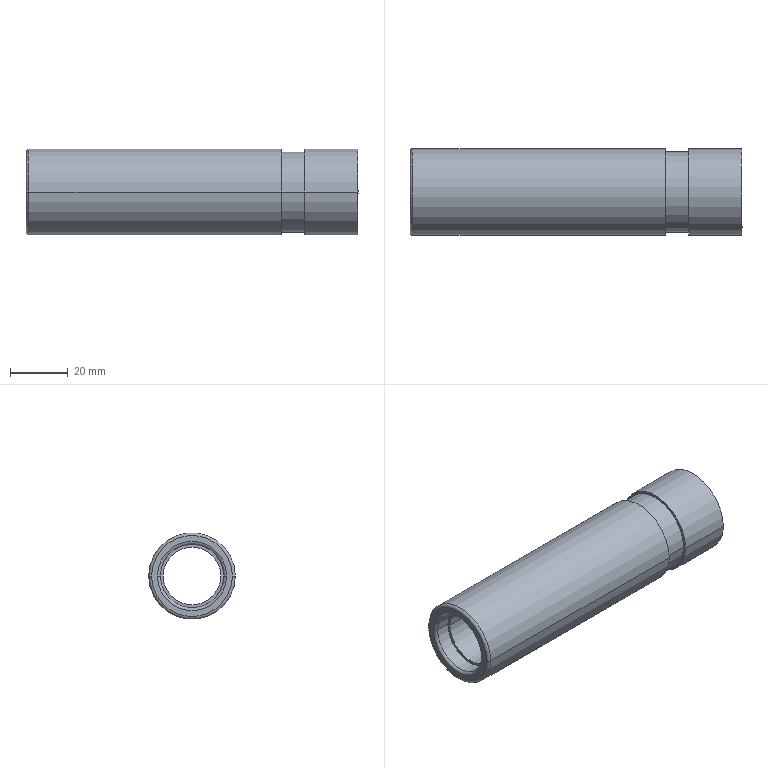Part | SolidWorks | features Fillet 1, Revolution 1 | 1 solid | 24 faces | box 115 x 30 x 30 mm | volume 43595 mm3 | cylinder 12 | torus 6 | plane 6 | commonest cylinder face diameters 30 x4 20 x2 21.974 x2 22 x2 28 x2
STEP:
#1=CARTESIAN_POINT('',(-54.57,8.757,0.));
#2=VERTEX_POINT('',#1);
#3=CARTESIAN_POINT('',(-54.57,-15.217,0.));
#4=VERTEX_POINT('',#3);
#5=CARTESIAN_POINT('',(-54.57,-3.23,0.));
#6=DIRECTION('',(1.,0.,0.));
#7=DIRECTION('',(0.,-1.,0.));
#8=AXIS2_PLACEMENT_3D('',#5,#6,#7);
#9=CIRCLE('',#8,11.987);
#10=EDGE_CURVE('',#2,#4,#9,.T.);
#11=ORIENTED_EDGE('',*,*,#10,.F.);
#12=CARTESIAN_POINT('',(-53.57,7.757,0.));
#13=VERTEX_POINT('',#12);
#14=CARTESIAN_POINT('',(-53.57,8.757,0.));
#15=DIRECTION('',(0.,0.,1.));
#16=DIRECTION('',(1.,0.,0.));
#17=AXIS2_PLACEMENT_3D('',#14,#15,#16);
#18=CIRCLE('',#17,1.);
#19=EDGE_CURVE('',#2,#13,#18,.T.);
#20=ORIENTED_EDGE('',*,*,#19,.T.);
#21=CARTESIAN_POINT('',(-53.57,-14.217,0.));
#22=VERTEX_POINT('',#21);
#23=CARTESIAN_POINT('',(-53.57,-3.23,0.));
#24=DIRECTION('',(-1.,0.,0.));
#25=DIRECTION('',(0.,-1.,0.));
#26=AXIS2_PLACEMENT_3D('',#23,#24,#25);
#27=CIRCLE('',#26,10.987);
#28=EDGE_CURVE('',#22,#13,#27,.T.);
#29=ORIENTED_EDGE('',*,*,#28,.F.);
#30=CARTESIAN_POINT('',(-53.57,-15.217,0.));
#31=DIRECTION('',(0.,0.,-1.));
#32=DIRECTION('',(-1.,0.,0.));
#33=AXIS2_PLACEMENT_3D('',#30,#31,#32);
#34=CIRCLE('',#33,1.);
#35=EDGE_CURVE('',#4,#22,#34,.T.);
#36=ORIENTED_EDGE('',*,*,#35,.F.);
#37=EDGE_LOOP('',(#11,#20,#29,#36));
#38=FACE_OUTER_BOUND('',#37,.T.);
#39=CARTESIAN_POINT('',(-53.57,-3.23,0.));
#40=DIRECTION('',(-1.,0.,0.));
#41=DIRECTION('',(0.,-1.,0.));
#42=AXIS2_PLACEMENT_3D('',#39,#40,#41);
#43=TOROIDAL_SURFACE('',#42,11.987,1.);
#44=ADVANCED_FACE('',(#38),#43,.T.);
#45=CARTESIAN_POINT('',(-53.57,11.77,0.));
#46=VERTEX_POINT('',#45);
#47=CARTESIAN_POINT('',(-53.57,-18.23,0.));
#48=VERTEX_POINT('',#47);
#49=CARTESIAN_POINT('',(-53.57,-3.23,0.));
#50=DIRECTION('',(1.,0.,0.));
#51=DIRECTION('',(0.,-1.,0.));
#52=AXIS2_PLACEMENT_3D('',#49,#50,#51);
#53=CIRCLE('',#52,15.);
#54=EDGE_CURVE('',#46,#48,#53,.T.);
#55=ORIENTED_EDGE('',*,*,#54,.F.);
#56=CARTESIAN_POINT('',(-54.57,10.77,0.));
#57=VERTEX_POINT('',#56);
#58=CARTESIAN_POINT('',(-53.57,10.77,0.));
#59=DIRECTION('',(0.,0.,1.));
#60=DIRECTION('',(1.,0.,0.));
#61=AXIS2_PLACEMENT_3D('',#58,#59,#60);
#62=CIRCLE('',#61,1.);
#63=EDGE_CURVE('',#46,#57,#62,.T.);
#64=ORIENTED_EDGE('',*,*,#63,.T.);
#65=CARTESIAN_POINT('',(-54.57,-17.23,0.));
#66=VERTEX_POINT('',#65);
#67=CARTESIAN_POINT('',(-54.57,-3.23,0.));
#68=DIRECTION('',(-1.,0.,0.));
#69=DIRECTION('',(0.,-1.,0.));
#70=AXIS2_PLACEMENT_3D('',#67,#68,#69);
#71=CIRCLE('',#70,14.);
#72=EDGE_CURVE('',#66,#57,#71,.T.);
#73=ORIENTED_EDGE('',*,*,#72,.F.);
#74=CARTESIAN_POINT('',(-53.57,-17.23,0.));
#75=DIRECTION('',(0.,0.,-1.));
#76=DIRECTION('',(-1.,0.,0.));
#77=AXIS2_PLACEMENT_3D('',#74,#75,#76);
#78=CIRCLE('',#77,1.);
#79=EDGE_CURVE('',#48,#66,#78,.T.);
#80=ORIENTED_EDGE('',*,*,#79,.F.);
#81=EDGE_LOOP('',(#55,#64,#73,#80));
#82=FACE_OUTER_BOUND('',#81,.T.);
#83=CARTESIAN_POINT('',(-53.57,-3.23,0.));
#84=DIRECTION('',(-1.,0.,0.));
#85=DIRECTION('',(0.,-1.,0.));
#86=AXIS2_PLACEMENT_3D('',#83,#84,#85);
#87=TOROIDAL_SURFACE('',#86,14.,1.);
#88=ADVANCED_FACE('',(#82),#87,.T.);
#89=CARTESIAN_POINT('',(60.43,-15.23,0.));
#90=VERTEX_POINT('',#89);
#91=CARTESIAN_POINT('',(60.43,8.77,0.));
#92=VERTEX_POINT('',#91);
#93=CARTESIAN_POINT('',(60.43,-3.23,0.));
#94=DIRECTION('',(-1.,0.,0.));
#95=DIRECTION('',(0.,1.,0.));
#96=AXIS2_PLACEMENT_3D('',#93,#94,#95);
#97=CIRCLE('',#96,12.);
#98=EDGE_CURVE('',#90,#92,#97,.T.);
#99=ORIENTED_EDGE('',*,*,#98,.F.);
#100=CARTESIAN_POINT('',(59.43,-14.23,0.));
#101=VERTEX_POINT('',#100);
#102=CARTESIAN_POINT('',(59.43,-15.23,0.));
#103=DIRECTION('',(0.,0.,1.));
#104=DIRECTION('',(1.,0.,0.));
#105=AXIS2_PLACEMENT_3D('',#102,#103,#104);
#106=CIRCLE('',#105,1.);
#107=EDGE_CURVE('',#90,#101,#106,.T.);
#108=ORIENTED_EDGE('',*,*,#107,.T.);
#109=CARTESIAN_POINT('',(59.43,7.77,0.));
#110=VERTEX_POINT('',#109);
#111=CARTESIAN_POINT('',(59.43,-3.23,0.));
#112=DIRECTION('',(1.,0.,0.));
#113=DIRECTION('',(0.,1.,0.));
#114=AXIS2_PLACEMENT_3D('',#111,#112,#113);
#115=CIRCLE('',#114,11.);
#116=EDGE_CURVE('',#110,#101,#115,.T.);
#117=ORIENTED_EDGE('',*,*,#116,.F.);
#118=CARTESIAN_POINT('',(59.43,8.77,0.));
#119=DIRECTION('',(0.,0.,-1.));
#120=DIRECTION('',(-1.,0.,0.));
#121=AXIS2_PLACEMENT_3D('',#118,#119,#120);
#122=CIRCLE('',#121,1.);
#123=EDGE_CURVE('',#92,#110,#122,.T.);
#124=ORIENTED_EDGE('',*,*,#123,.F.);
#125=EDGE_LOOP('',(#99,#108,#117,#124));
#126=FACE_OUTER_BOUND('',#125,.T.);
#127=CARTESIAN_POINT('',(59.43,-3.23,0.));
#128=DIRECTION('',(1.,0.,0.));
#129=DIRECTION('',(0.,1.,0.));
#130=AXIS2_PLACEMENT_3D('',#127,#128,#129);
#131=TOROIDAL_SURFACE('',#130,12.,1.);
#132=ADVANCED_FACE('',(#126),#131,.T.);
#133=CARTESIAN_POINT('',(33.93,10.77,0.));
#134=VERTEX_POINT('',#133);
#135=CARTESIAN_POINT('',(33.93,-17.23,0.));
#136=VERTEX_POINT('',#135);
#137=CARTESIAN_POINT('',(33.93,-3.23,0.));
#138=DIRECTION('',(1.,0.,0.));
#139=DIRECTION('',(0.,1.,0.));
#140=AXIS2_PLACEMENT_3D('',#137,#138,#139);
#141=CIRCLE('',#140,14.);
#142=EDGE_CURVE('',#134,#136,#141,.T.);
#143=ORIENTED_EDGE('',*,*,#142,.T.);
#144=CARTESIAN_POINT('',(41.93,-17.23,0.));
#145=VERTEX_POINT('',#144);
#146=CARTESIAN_POINT('',(54.43,-17.23,0.));
#147=DIRECTION('',(1.,0.,0.));
#148=VECTOR('',#147,1000.);
#149=LINE('',#146,#148);
#150=EDGE_CURVE('',#136,#145,#149,.T.);
#151=ORIENTED_EDGE('',*,*,#150,.T.);
#152=CARTESIAN_POINT('',(41.93,10.77,0.));
#153=VERTEX_POINT('',#152);
#154=CARTESIAN_POINT('',(41.93,-3.23,0.));
#155=DIRECTION('',(1.,0.,0.));
#156=DIRECTION('',(0.,1.,0.));
#157=AXIS2_PLACEMENT_3D('',#154,#155,#156);
#158=CIRCLE('',#157,14.);
#159=EDGE_CURVE('',#153,#145,#158,.T.);
#160=ORIENTED_EDGE('',*,*,#159,.F.);
#161=CARTESIAN_POINT('',(54.43,10.77,0.));
#162=DIRECTION('',(1.,0.,0.));
#163=VECTOR('',#162,1000.);
#164=LINE('',#161,#163);
#165=EDGE_CURVE('',#134,#153,#164,.T.);
#166=ORIENTED_EDGE('',*,*,#165,.F.);
#167=EDGE_LOOP('',(#143,#151,#160,#166));
#168=FACE_OUTER_BOUND('',#167,.T.);
#169=CARTESIAN_POINT('',(54.43,-3.23,0.));
#170=DIRECTION('',(1.,0.,0.));
#171=DIRECTION('',(0.,1.,0.));
#172=AXIS2_PLACEMENT_3D('',#169,#170,#171);
#173=CYLINDRICAL_SURFACE('',#172,14.);
#174=ADVANCED_FACE('',(#168),#173,.T.);
#175=ORIENTED_EDGE('',*,*,#54,.T.);
#176=CARTESIAN_POINT('',(33.93,-18.23,0.));
#177=VERTEX_POINT('',#176);
#178=CARTESIAN_POINT('',(54.43,-18.23,0.));
#179=DIRECTION('',(1.,0.,0.));
#180=VECTOR('',#179,1000.);
#181=LINE('',#178,#180);
#182=EDGE_CURVE('',#48,#177,#181,.T.);
#183=ORIENTED_EDGE('',*,*,#182,.T.);
#184=CARTESIAN_POINT('',(33.93,11.77,0.));
#185=VERTEX_POINT('',#184);
#186=CARTESIAN_POINT('',(33.93,-3.23,0.));
#187=DIRECTION('',(1.,0.,0.));
#188=DIRECTION('',(0.,1.,0.));
#189=AXIS2_PLACEMENT_3D('',#186,#187,#188);
#190=CIRCLE('',#189,15.);
#191=EDGE_CURVE('',#185,#177,#190,.T.);
#192=ORIENTED_EDGE('',*,*,#191,.F.);
#193=CARTESIAN_POINT('',(54.43,11.77,0.));
#194=DIRECTION('',(1.,0.,0.));
#195=VECTOR('',#194,1000.);
#196=LINE('',#193,#195);
#197=EDGE_CURVE('',#46,#185,#196,.T.);
#198=ORIENTED_EDGE('',*,*,#197,.F.);
#199=EDGE_LOOP('',(#175,#183,#192,#198));
#200=FACE_OUTER_BOUND('',#199,.T.);
#201=CARTESIAN_POINT('',(54.43,-3.23,0.));
#202=DIRECTION('',(1.,0.,0.));
#203=DIRECTION('',(0.,1.,0.));
#204=AXIS2_PLACEMENT_3D('',#201,#202,#203);
#205=CYLINDRICAL_SURFACE('',#204,15.);
#206=ADVANCED_FACE('',(#200),#205,.T.);
#207=CARTESIAN_POINT('',(-53.57,-3.23,0.));
#208=DIRECTION('',(-1.,0.,0.));
#209=DIRECTION('',(0.,-1.,0.));
#210=AXIS2_PLACEMENT_3D('',#207,#208,#209);
#211=CIRCLE('',#210,10.987);
#212=EDGE_CURVE('',#13,#22,#211,.T.);
#213=ORIENTED_EDGE('',*,*,#212,.T.);
#214=CARTESIAN_POINT('',(-48.57,-14.217,0.));
#215=VERTEX_POINT('',#214);
#216=CARTESIAN_POINT('',(54.43,-14.217,0.));
#217=DIRECTION('',(1.,0.,0.));
#218=VECTOR('',#217,1000.);
#219=LINE('',#216,#218);
#220=EDGE_CURVE('',#22,#215,#219,.T.);
#221=ORIENTED_EDGE('',*,*,#220,.T.);
#222=CARTESIAN_POINT('',(-48.57,7.757,0.));
#223=VERTEX_POINT('',#222);
#224=CARTESIAN_POINT('',(-48.57,-3.23,0.));
#225=DIRECTION('',(1.,0.,0.));
#226=DIRECTION('',(0.,1.,0.));
#227=AXIS2_PLACEMENT_3D('',#224,#225,#226);
#228=CIRCLE('',#227,10.987);
#229=EDGE_CURVE('',#215,#223,#228,.T.);
#230=ORIENTED_EDGE('',*,*,#229,.T.);
#231=CARTESIAN_POINT('',(54.43,7.757,0.));
#232=DIRECTION('',(1.,0.,0.));
#233=VECTOR('',#232,1000.);
#234=LINE('',#231,#233);
#235=EDGE_CURVE('',#13,#223,#234,.T.);
#236=ORIENTED_EDGE('',*,*,#235,.F.);
#237=EDGE_LOOP('',(#213,#221,#230,#236));
#238=FACE_OUTER_BOUND('',#237,.T.);
#239=CARTESIAN_POINT('',(54.43,-3.23,0.));
#240=DIRECTION('',(1.,0.,0.));
#241=DIRECTION('',(0.,1.,0.));
#242=AXIS2_PLACEMENT_3D('',#239,#240,#241);
#243=CYLINDRICAL_SURFACE('',#242,10.987);
#244=ADVANCED_FACE('',(#238),#243,.F.);
#245=CARTESIAN_POINT('',(-48.57,-13.23,0.));
#246=VERTEX_POINT('',#245);
#247=CARTESIAN_POINT('',(-48.57,6.77,0.));
#248=VERTEX_POINT('',#247);
#249=CARTESIAN_POINT('',(-48.57,-3.23,0.));
#250=DIRECTION('',(1.,0.,0.));
#251=DIRECTION('',(0.,1.,0.));
#252=AXIS2_PLACEMENT_3D('',#249,#250,#251);
#253=CIRCLE('',#252,10.);
#254=EDGE_CURVE('',#246,#248,#253,.T.);
#255=ORIENTED_EDGE('',*,*,#254,.F.);
#256=CARTESIAN_POINT('',(54.43,-13.23,0.));
#257=VERTEX_POINT('',#256);
#258=CARTESIAN_POINT('',(54.43,-13.23,0.));
#259=DIRECTION('',(1.,0.,0.));
#260=VECTOR('',#259,1000.);
#261=LINE('',#258,#260);
#262=EDGE_CURVE('',#246,#257,#261,.T.);
#263=ORIENTED_EDGE('',*,*,#262,.T.);
#264=CARTESIAN_POINT('',(54.43,6.77,0.));
#265=VERTEX_POINT('',#264);
#266=CARTESIAN_POINT('',(54.43,-3.23,0.));
#267=DIRECTION('',(1.,0.,0.));
#268=DIRECTION('',(0.,1.,0.));
#269=AXIS2_PLACEMENT_3D('',#266,#267,#268);
#270=CIRCLE('',#269,10.);
#271=EDGE_CURVE('',#257,#265,#270,.T.);
#272=ORIENTED_EDGE('',*,*,#271,.T.);
#273=CARTESIAN_POINT('',(54.43,6.77,0.));
#274=DIRECTION('',(1.,0.,0.));
#275=VECTOR('',#274,1000.);
#276=LINE('',#273,#275);
#277=EDGE_CURVE('',#248,#265,#276,.T.);
#278=ORIENTED_EDGE('',*,*,#277,.F.);
#279=EDGE_LOOP('',(#255,#263,#272,#278));
#280=FACE_OUTER_BOUND('',#279,.T.);
#281=CARTESIAN_POINT('',(54.43,-3.23,0.));
#282=DIRECTION('',(1.,0.,0.));
#283=DIRECTION('',(0.,1.,0.));
#284=AXIS2_PLACEMENT_3D('',#281,#282,#283);
#285=CYLINDRICAL_SURFACE('',#284,10.);
#286=ADVANCED_FACE('',(#280),#285,.F.);
#287=CARTESIAN_POINT('',(54.43,-14.23,0.));
#288=VERTEX_POINT('',#287);
#289=CARTESIAN_POINT('',(54.43,7.77,0.));
#290=VERTEX_POINT('',#289);
#291=CARTESIAN_POINT('',(54.43,-3.23,0.));
#292=DIRECTION('',(1.,0.,0.));
#293=DIRECTION('',(0.,1.,0.));
#294=AXIS2_PLACEMENT_3D('',#291,#292,#293);
#295=CIRCLE('',#294,11.);
#296=EDGE_CURVE('',#288,#290,#295,.T.);
#297=ORIENTED_EDGE('',*,*,#296,.F.);
#298=CARTESIAN_POINT('',(54.43,-14.23,0.));
#299=DIRECTION('',(1.,0.,0.));
#300=VECTOR('',#299,1000.);
#301=LINE('',#298,#300);
#302=EDGE_CURVE('',#288,#101,#301,.T.);
#303=ORIENTED_EDGE('',*,*,#302,.T.);
#304=CARTESIAN_POINT('',(59.43,-3.23,0.));
#305=DIRECTION('',(1.,0.,0.));
#306=DIRECTION('',(0.,1.,0.));
#307=AXIS2_PLACEMENT_3D('',#304,#305,#306);
#308=CIRCLE('',#307,11.);
#309=EDGE_CURVE('',#101,#110,#308,.T.);
#310=ORIENTED_EDGE('',*,*,#309,.T.);
#311=CARTESIAN_POINT('',(54.43,7.77,0.));
#312=DIRECTION('',(1.,0.,0.));
#313=VECTOR('',#312,1000.);
#314=LINE('',#311,#313);
#315=EDGE_CURVE('',#290,#110,#314,.T.);
#316=ORIENTED_EDGE('',*,*,#315,.F.);
#317=EDGE_LOOP('',(#297,#303,#310,#316));
#318=FACE_OUTER_BOUND('',#317,.T.);
#319=CARTESIAN_POINT('',(54.43,-3.23,0.));
#320=DIRECTION('',(1.,0.,0.));
#321=DIRECTION('',(0.,1.,0.));
#322=AXIS2_PLACEMENT_3D('',#319,#320,#321);
#323=CYLINDRICAL_SURFACE('',#322,11.);
#324=ADVANCED_FACE('',(#318),#323,.F.);
#325=CARTESIAN_POINT('',(41.93,11.77,0.));
#326=VERTEX_POINT('',#325);
#327=CARTESIAN_POINT('',(41.93,-18.23,0.));
#328=VERTEX_POINT('',#327);
#329=CARTESIAN_POINT('',(41.93,-3.23,0.));
#330=DIRECTION('',(1.,0.,0.));
#331=DIRECTION('',(0.,1.,0.));
#332=AXIS2_PLACEMENT_3D('',#329,#330,#331);
#333=CIRCLE('',#332,15.);
#334=EDGE_CURVE('',#326,#328,#333,.T.);
#335=ORIENTED_EDGE('',*,*,#334,.T.);
#336=CARTESIAN_POINT('',(60.43,-18.23,0.));
#337=VERTEX_POINT('',#336);
#338=CARTESIAN_POINT('',(54.43,-18.23,0.));
#339=DIRECTION('',(1.,0.,0.));
#340=VECTOR('',#339,1000.);
#341=LINE('',#338,#340);
#342=EDGE_CURVE('',#328,#337,#341,.T.);
#343=ORIENTED_EDGE('',*,*,#342,.T.);
#344=CARTESIAN_POINT('',(60.43,11.77,0.));
#345=VERTEX_POINT('',#344);
#346=CARTESIAN_POINT('',(60.43,-3.23,0.));
#347=DIRECTION('',(1.,0.,0.));
#348=DIRECTION('',(0.,1.,0.));
#349=AXIS2_PLACEMENT_3D('',#346,#347,#348);
#350=CIRCLE('',#349,15.);
#351=EDGE_CURVE('',#345,#337,#350,.T.);
#352=ORIENTED_EDGE('',*,*,#351,.F.);
#353=CARTESIAN_POINT('',(54.43,11.77,0.));
#354=DIRECTION('',(1.,0.,0.));
#355=VECTOR('',#354,1000.);
#356=LINE('',#353,#355);
#357=EDGE_CURVE('',#326,#345,#356,.T.);
#358=ORIENTED_EDGE('',*,*,#357,.F.);
#359=EDGE_LOOP('',(#335,#343,#352,#358));
#360=FACE_OUTER_BOUND('',#359,.T.);
#361=CARTESIAN_POINT('',(54.43,-3.23,0.));
#362=DIRECTION('',(1.,0.,0.));
#363=DIRECTION('',(0.,1.,0.));
#364=AXIS2_PLACEMENT_3D('',#361,#362,#363);
#365=CYLINDRICAL_SURFACE('',#364,15.);
#366=ADVANCED_FACE('',(#360),#365,.T.);
#367=ORIENTED_EDGE('',*,*,#342,.F.);
#368=CARTESIAN_POINT('',(41.93,-3.23,0.));
#369=DIRECTION('',(1.,0.,0.));
#370=DIRECTION('',(0.,1.,0.));
#371=AXIS2_PLACEMENT_3D('',#368,#369,#370);
#372=CIRCLE('',#371,15.);
#373=EDGE_CURVE('',#328,#326,#372,.T.);
#374=ORIENTED_EDGE('',*,*,#373,.T.);
#375=ORIENTED_EDGE('',*,*,#357,.T.);
#376=CARTESIAN_POINT('',(60.43,-3.23,0.));
#377=DIRECTION('',(1.,0.,0.));
#378=DIRECTION('',(0.,1.,0.));
#379=AXIS2_PLACEMENT_3D('',#376,#377,#378);
#380=CIRCLE('',#379,15.);
#381=EDGE_CURVE('',#337,#345,#380,.T.);
#382=ORIENTED_EDGE('',*,*,#381,.F.);
#383=EDGE_LOOP('',(#367,#374,#375,#382));
#384=FACE_OUTER_BOUND('',#383,.T.);
#385=CARTESIAN_POINT('',(54.43,-3.23,0.));
#386=DIRECTION('',(1.,0.,0.));
#387=DIRECTION('',(0.,1.,0.));
#388=AXIS2_PLACEMENT_3D('',#385,#386,#387);
#389=CYLINDRICAL_SURFACE('',#388,15.);
#390=ADVANCED_FACE('',(#384),#389,.T.);
#391=CARTESIAN_POINT('',(60.43,-3.23,0.));
#392=DIRECTION('',(-1.,0.,0.));
#393=DIRECTION('',(0.,1.,0.));
#394=AXIS2_PLACEMENT_3D('',#391,#392,#393);
#395=CIRCLE('',#394,12.);
#396=EDGE_CURVE('',#92,#90,#395,.T.);
#397=ORIENTED_EDGE('',*,*,#396,.T.);
#398=ORIENTED_EDGE('',*,*,#98,.T.);
#399=EDGE_LOOP('',(#397,#398));
#400=FACE_BOUND('',#399,.T.);
#401=ORIENTED_EDGE('',*,*,#351,.T.);
#402=ORIENTED_EDGE('',*,*,#381,.T.);
#403=EDGE_LOOP('',(#401,#402));
#404=FACE_OUTER_BOUND('',#403,.T.);
#405=CARTESIAN_POINT('',(60.43,11.77,0.));
#406=DIRECTION('',(1.,0.,0.));
#407=DIRECTION('',(0.,1.,0.));
#408=AXIS2_PLACEMENT_3D('',#405,#406,#407);
#409=PLANE('',#408);
#410=ADVANCED_FACE('',(#400,#404),#409,.T.);
#411=ORIENTED_EDGE('',*,*,#302,.F.);
#412=CARTESIAN_POINT('',(54.43,-3.23,0.));
#413=DIRECTION('',(1.,0.,0.));
#414=DIRECTION('',(0.,1.,0.));
#415=AXIS2_PLACEMENT_3D('',#412,#413,#414);
#416=CIRCLE('',#415,11.);
#417=EDGE_CURVE('',#290,#288,#416,.T.);
#418=ORIENTED_EDGE('',*,*,#417,.F.);
#419=ORIENTED_EDGE('',*,*,#315,.T.);
#420=ORIENTED_EDGE('',*,*,#116,.T.);
#421=EDGE_LOOP('',(#411,#418,#419,#420));
#422=FACE_OUTER_BOUND('',#421,.T.);
#423=CARTESIAN_POINT('',(54.43,-3.23,0.));
#424=DIRECTION('',(1.,0.,0.));
#425=DIRECTION('',(0.,1.,0.));
#426=AXIS2_PLACEMENT_3D('',#423,#424,#425);
#427=CYLINDRICAL_SURFACE('',#426,11.);
#428=ADVANCED_FACE('',(#422),#427,.F.);
#429=ORIENTED_EDGE('',*,*,#417,.T.);
#430=ORIENTED_EDGE('',*,*,#296,.T.);
#431=EDGE_LOOP('',(#429,#430));
#432=FACE_OUTER_BOUND('',#431,.T.);
#433=CARTESIAN_POINT('',(54.43,-3.23,0.));
#434=DIRECTION('',(1.,0.,0.));
#435=DIRECTION('',(0.,1.,0.));
#436=AXIS2_PLACEMENT_3D('',#433,#434,#435);
#437=CIRCLE('',#436,10.);
#438=EDGE_CURVE('',#265,#257,#437,.T.);
#439=ORIENTED_EDGE('',*,*,#438,.F.);
#440=ORIENTED_EDGE('',*,*,#271,.F.);
#441=EDGE_LOOP('',(#439,#440));
#442=FACE_BOUND('',#441,.T.);
#443=CARTESIAN_POINT('',(54.43,7.77,0.));
#444=DIRECTION('',(1.,0.,0.));
#445=DIRECTION('',(0.,1.,0.));
#446=AXIS2_PLACEMENT_3D('',#443,#444,#445);
#447=PLANE('',#446);
#448=ADVANCED_FACE('',(#432,#442),#447,.T.);
#449=ORIENTED_EDGE('',*,*,#262,.F.);
#450=CARTESIAN_POINT('',(-48.57,-3.23,0.));
#451=DIRECTION('',(1.,0.,0.));
#452=DIRECTION('',(0.,1.,0.));
#453=AXIS2_PLACEMENT_3D('',#450,#451,#452);
#454=CIRCLE('',#453,10.);
#455=EDGE_CURVE('',#248,#246,#454,.T.);
#456=ORIENTED_EDGE('',*,*,#455,.F.);
#457=ORIENTED_EDGE('',*,*,#277,.T.);
#458=ORIENTED_EDGE('',*,*,#438,.T.);
#459=EDGE_LOOP('',(#449,#456,#457,#458));
#460=FACE_OUTER_BOUND('',#459,.T.);
#461=CARTESIAN_POINT('',(54.43,-3.23,0.));
#462=DIRECTION('',(1.,0.,0.));
#463=DIRECTION('',(0.,1.,0.));
#464=AXIS2_PLACEMENT_3D('',#461,#462,#463);
#465=CYLINDRICAL_SURFACE('',#464,10.);
#466=ADVANCED_FACE('',(#460),#465,.F.);
#467=ORIENTED_EDGE('',*,*,#455,.T.);
#468=ORIENTED_EDGE('',*,*,#254,.T.);
#469=EDGE_LOOP('',(#467,#468));
#470=FACE_BOUND('',#469,.T.);
#471=CARTESIAN_POINT('',(-48.57,-3.23,0.));
#472=DIRECTION('',(1.,0.,0.));
#473=DIRECTION('',(0.,1.,0.));
#474=AXIS2_PLACEMENT_3D('',#471,#472,#473);
#475=CIRCLE('',#474,10.987);
#476=EDGE_CURVE('',#223,#215,#475,.T.);
#477=ORIENTED_EDGE('',*,*,#476,.F.);
#478=ORIENTED_EDGE('',*,*,#229,.F.);
#479=EDGE_LOOP('',(#477,#478));
#480=FACE_OUTER_BOUND('',#479,.T.);
#481=CARTESIAN_POINT('',(-48.57,7.757,0.));
#482=DIRECTION('',(-1.,0.,0.));
#483=DIRECTION('',(0.,-1.,0.));
#484=AXIS2_PLACEMENT_3D('',#481,#482,#483);
#485=PLANE('',#484);
#486=ADVANCED_FACE('',(#470,#480),#485,.T.);
#487=ORIENTED_EDGE('',*,*,#220,.F.);
#488=ORIENTED_EDGE('',*,*,#28,.T.);
#489=ORIENTED_EDGE('',*,*,#235,.T.);
#490=ORIENTED_EDGE('',*,*,#476,.T.);
#491=EDGE_LOOP('',(#487,#488,#489,#490));
#492=FACE_OUTER_BOUND('',#491,.T.);
#493=CARTESIAN_POINT('',(54.43,-3.23,0.));
#494=DIRECTION('',(1.,0.,0.));
#495=DIRECTION('',(0.,1.,0.));
#496=AXIS2_PLACEMENT_3D('',#493,#494,#495);
#497=CYLINDRICAL_SURFACE('',#496,10.987);
#498=ADVANCED_FACE('',(#492),#497,.F.);
#499=ORIENTED_EDGE('',*,*,#72,.T.);
#500=CARTESIAN_POINT('',(-54.57,-3.23,0.));
#501=DIRECTION('',(-1.,0.,0.));
#502=DIRECTION('',(0.,-1.,0.));
#503=AXIS2_PLACEMENT_3D('',#500,#501,#502);
#504=CIRCLE('',#503,14.);
#505=EDGE_CURVE('',#57,#66,#504,.T.);
#506=ORIENTED_EDGE('',*,*,#505,.T.);
#507=EDGE_LOOP('',(#499,#506));
#508=FACE_OUTER_BOUND('',#507,.T.);
#509=CARTESIAN_POINT('',(-54.57,-3.23,0.));
#510=DIRECTION('',(1.,0.,0.));
#511=DIRECTION('',(0.,-1.,0.));
#512=AXIS2_PLACEMENT_3D('',#509,#510,#511);
#513=CIRCLE('',#512,11.987);
#514=EDGE_CURVE('',#4,#2,#513,.T.);
#515=ORIENTED_EDGE('',*,*,#514,.T.);
#516=ORIENTED_EDGE('',*,*,#10,.T.);
#517=EDGE_LOOP('',(#515,#516));
#518=FACE_BOUND('',#517,.T.);
#519=CARTESIAN_POINT('',(-54.57,7.757,0.));
#520=DIRECTION('',(-1.,0.,0.));
#521=DIRECTION('',(0.,-1.,0.));
#522=AXIS2_PLACEMENT_3D('',#519,#520,#521);
#523=PLANE('',#522);
#524=ADVANCED_FACE('',(#508,#518),#523,.T.);
#525=ORIENTED_EDGE('',*,*,#182,.F.);
#526=CARTESIAN_POINT('',(-53.57,-3.23,0.));
#527=DIRECTION('',(1.,0.,0.));
#528=DIRECTION('',(0.,-1.,0.));
#529=AXIS2_PLACEMENT_3D('',#526,#527,#528);
#530=CIRCLE('',#529,15.);
#531=EDGE_CURVE('',#48,#46,#530,.T.);
#532=ORIENTED_EDGE('',*,*,#531,.T.);
#533=ORIENTED_EDGE('',*,*,#197,.T.);
#534=CARTESIAN_POINT('',(33.93,-3.23,0.));
#535=DIRECTION('',(1.,0.,0.));
#536=DIRECTION('',(0.,1.,0.));
#537=AXIS2_PLACEMENT_3D('',#534,#535,#536);
#538=CIRCLE('',#537,15.);
#539=EDGE_CURVE('',#177,#185,#538,.T.);
#540=ORIENTED_EDGE('',*,*,#539,.F.);
#541=EDGE_LOOP('',(#525,#532,#533,#540));
#542=FACE_OUTER_BOUND('',#541,.T.);
#543=CARTESIAN_POINT('',(54.43,-3.23,0.));
#544=DIRECTION('',(1.,0.,0.));
#545=DIRECTION('',(0.,1.,0.));
#546=AXIS2_PLACEMENT_3D('',#543,#544,#545);
#547=CYLINDRICAL_SURFACE('',#546,15.);
#548=ADVANCED_FACE('',(#542),#547,.T.);
#549=ORIENTED_EDGE('',*,*,#191,.T.);
#550=ORIENTED_EDGE('',*,*,#539,.T.);
#551=EDGE_LOOP('',(#549,#550));
#552=FACE_OUTER_BOUND('',#551,.T.);
#553=ORIENTED_EDGE('',*,*,#142,.F.);
#554=CARTESIAN_POINT('',(33.93,-3.23,0.));
#555=DIRECTION('',(1.,0.,0.));
#556=DIRECTION('',(0.,1.,0.));
#557=AXIS2_PLACEMENT_3D('',#554,#555,#556);
#558=CIRCLE('',#557,14.);
#559=EDGE_CURVE('',#136,#134,#558,.T.);
#560=ORIENTED_EDGE('',*,*,#559,.F.);
#561=EDGE_LOOP('',(#553,#560));
#562=FACE_BOUND('',#561,.T.);
#563=CARTESIAN_POINT('',(33.93,10.77,0.));
#564=DIRECTION('',(1.,0.,0.));
#565=DIRECTION('',(0.,1.,0.));
#566=AXIS2_PLACEMENT_3D('',#563,#564,#565);
#567=PLANE('',#566);
#568=ADVANCED_FACE('',(#552,#562),#567,.T.);
#569=ORIENTED_EDGE('',*,*,#150,.F.);
#570=ORIENTED_EDGE('',*,*,#559,.T.);
#571=ORIENTED_EDGE('',*,*,#165,.T.);
#572=CARTESIAN_POINT('',(41.93,-3.23,0.));
#573=DIRECTION('',(1.,0.,0.));
#574=DIRECTION('',(0.,1.,0.));
#575=AXIS2_PLACEMENT_3D('',#572,#573,#574);
#576=CIRCLE('',#575,14.);
#577=EDGE_CURVE('',#145,#153,#576,.T.);
#578=ORIENTED_EDGE('',*,*,#577,.F.);
#579=EDGE_LOOP('',(#569,#570,#571,#578));
#580=FACE_OUTER_BOUND('',#579,.T.);
#581=CARTESIAN_POINT('',(54.43,-3.23,0.));
#582=DIRECTION('',(1.,0.,0.));
#583=DIRECTION('',(0.,1.,0.));
#584=AXIS2_PLACEMENT_3D('',#581,#582,#583);
#585=CYLINDRICAL_SURFACE('',#584,14.);
#586=ADVANCED_FACE('',(#580),#585,.T.);
#587=ORIENTED_EDGE('',*,*,#159,.T.);
#588=ORIENTED_EDGE('',*,*,#577,.T.);
#589=EDGE_LOOP('',(#587,#588));
#590=FACE_BOUND('',#589,.T.);
#591=ORIENTED_EDGE('',*,*,#334,.F.);
#592=ORIENTED_EDGE('',*,*,#373,.F.);
#593=EDGE_LOOP('',(#591,#592));
#594=FACE_OUTER_BOUND('',#593,.T.);
#595=CARTESIAN_POINT('',(41.93,11.77,0.));
#596=DIRECTION('',(-1.,0.,0.));
#597=DIRECTION('',(0.,-1.,0.));
#598=AXIS2_PLACEMENT_3D('',#595,#596,#597);
#599=PLANE('',#598);
#600=ADVANCED_FACE('',(#590,#594),#599,.T.);
#601=ORIENTED_EDGE('',*,*,#107,.F.);
#602=ORIENTED_EDGE('',*,*,#396,.F.);
#603=ORIENTED_EDGE('',*,*,#123,.T.);
#604=ORIENTED_EDGE('',*,*,#309,.F.);
#605=EDGE_LOOP('',(#601,#602,#603,#604));
#606=FACE_OUTER_BOUND('',#605,.T.);
#607=CARTESIAN_POINT('',(59.43,-3.23,0.));
#608=DIRECTION('',(1.,0.,0.));
#609=DIRECTION('',(0.,1.,0.));
#610=AXIS2_PLACEMENT_3D('',#607,#608,#609);
#611=TOROIDAL_SURFACE('',#610,12.,1.);
#612=ADVANCED_FACE('',(#606),#611,.T.);
#613=ORIENTED_EDGE('',*,*,#63,.F.);
#614=ORIENTED_EDGE('',*,*,#531,.F.);
#615=ORIENTED_EDGE('',*,*,#79,.T.);
#616=ORIENTED_EDGE('',*,*,#505,.F.);
#617=EDGE_LOOP('',(#613,#614,#615,#616));
#618=FACE_OUTER_BOUND('',#617,.T.);
#619=CARTESIAN_POINT('',(-53.57,-3.23,0.));
#620=DIRECTION('',(-1.,0.,0.));
#621=DIRECTION('',(0.,-1.,0.));
#622=AXIS2_PLACEMENT_3D('',#619,#620,#621);
#623=TOROIDAL_SURFACE('',#622,14.,1.);
#624=ADVANCED_FACE('',(#618),#623,.T.);
#625=ORIENTED_EDGE('',*,*,#19,.F.);
#626=ORIENTED_EDGE('',*,*,#514,.F.);
#627=ORIENTED_EDGE('',*,*,#35,.T.);
#628=ORIENTED_EDGE('',*,*,#212,.F.);
#629=EDGE_LOOP('',(#625,#626,#627,#628));
#630=FACE_OUTER_BOUND('',#629,.T.);
#631=CARTESIAN_POINT('',(-53.57,-3.23,0.));
#632=DIRECTION('',(-1.,0.,0.));
#633=DIRECTION('',(0.,-1.,0.));
#634=AXIS2_PLACEMENT_3D('',#631,#632,#633);
#635=TOROIDAL_SURFACE('',#634,11.987,1.);
#636=ADVANCED_FACE('',(#630),#635,.T.);
#637=CLOSED_SHELL('',(#44,#88,#132,#174,#206,#244,#286,#324,#366,#390,#410,#428,#448,#466,#486,#498,#524,#548,#568,#586,#600,#612,#624,#636));
#638=MANIFOLD_SOLID_BREP('',#637);
#639=CARTESIAN_POINT('',(0.,0.,0.));
#640=DIRECTION('',(0.,0.,1.));
#641=DIRECTION('',(1.,0.,0.));
#642=AXIS2_PLACEMENT_3D('',#639,#640,#641);
#643=(LENGTH_UNIT()NAMED_UNIT(*)SI_UNIT(.MILLI.,.METRE.));
#644=UNCERTAINTY_MEASURE_WITH_UNIT(LENGTH_MEASURE(0.00001),#643,'','');
#645=(NAMED_UNIT(*)PLANE_ANGLE_UNIT()SI_UNIT($,.RADIAN.));
#646=(NAMED_UNIT(*)SI_UNIT($,.STERADIAN.)SOLID_ANGLE_UNIT());
#647=(GEOMETRIC_REPRESENTATION_CONTEXT(3)GLOBAL_UNCERTAINTY_ASSIGNED_CONTEXT((#644))GLOBAL_UNIT_ASSIGNED_CONTEXT((#643,#645,#646))REPRESENTATION_CONTEXT('',''));
#648=ADVANCED_BREP_SHAPE_REPRESENTATION('',(#638,#642),#647);